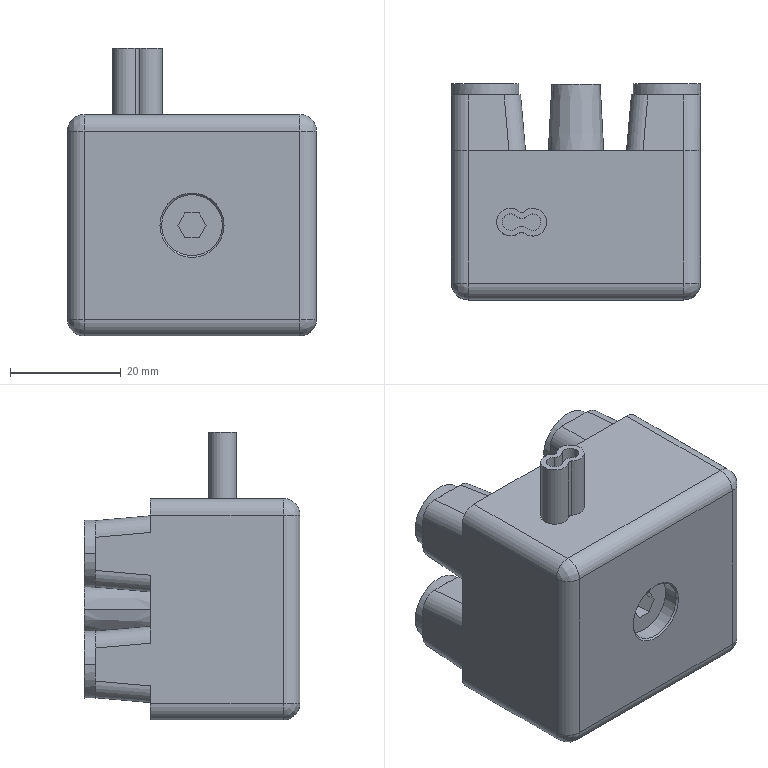Part | STEP file | BRACKET-none | 1 solid | 115 faces | box 45 x 39 x 52 mm | volume 53167 mm3 | plane 57 | cylinder 50 | other 4 | cone 4 | commonest cylinder face diameters 6 x24 6.8 x8 12.2 x8 3 x2 5 x2 11 x2